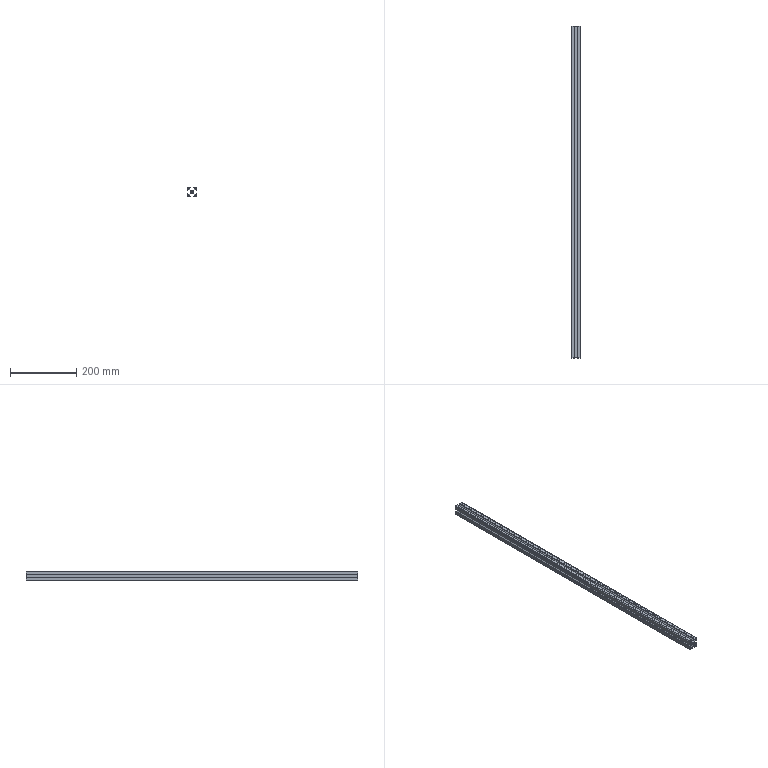Part | SolidWorks | features Extrusion 1 | 1 solid | 60 faces | box 30 x 1000 x 30 mm | volume 332538 mm3 | plane 46 | cylinder 14 | commonest cylinder face diameters 4.2 x8 4 x4 6.8 x2